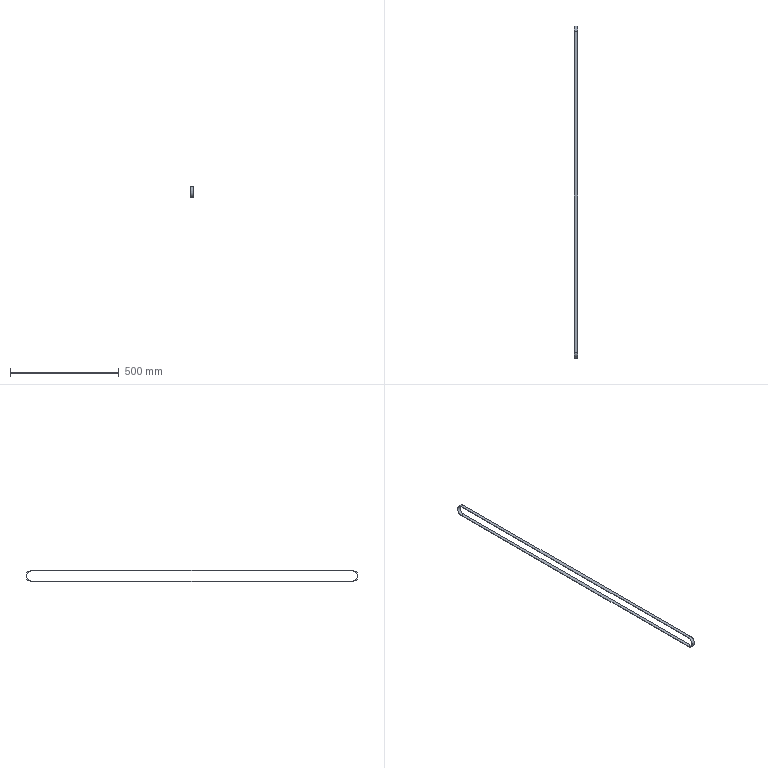Part | SolidWorks | features BaseBody 1 | 1 solid | 10 faces | box 15 x 1524 x 50.9 mm | volume 92989 mm3 | plane 6 | cylinder 4 | commonest cylinder face diameters 46.9 x2 50.9 x2
STEP:
#1=CARTESIAN_POINT('',(32.847,1932.,-322.55));
#2=VERTEX_POINT('',#1);
#3=CARTESIAN_POINT('',(32.847,459.,-322.55));
#4=VERTEX_POINT('',#3);
#5=CARTESIAN_POINT('',(32.847,1982.,-322.55));
#6=DIRECTION('',(0.,-1.,0.));
#7=VECTOR('',#6,1000.);
#8=LINE('',#5,#7);
#9=EDGE_CURVE('',#2,#4,#8,.T.);
#10=ORIENTED_EDGE('',*,*,#9,.F.);
#11=CARTESIAN_POINT('',(17.847,1932.,-322.55));
#12=VERTEX_POINT('',#11);
#13=CARTESIAN_POINT('',(32.847,1932.,-322.55));
#14=DIRECTION('',(1.,0.,0.));
#15=VECTOR('',#14,1000.);
#16=LINE('',#13,#15);
#17=EDGE_CURVE('',#12,#2,#16,.T.);
#18=ORIENTED_EDGE('',*,*,#17,.F.);
#19=CARTESIAN_POINT('',(17.847,459.,-322.55));
#20=VERTEX_POINT('',#19);
#21=CARTESIAN_POINT('',(17.847,1982.,-322.55));
#22=DIRECTION('',(0.,1.,0.));
#23=VECTOR('',#22,1000.);
#24=LINE('',#21,#23);
#25=EDGE_CURVE('',#20,#12,#24,.T.);
#26=ORIENTED_EDGE('',*,*,#25,.F.);
#27=CARTESIAN_POINT('',(32.847,459.,-322.55));
#28=DIRECTION('',(-1.,0.,0.));
#29=VECTOR('',#28,1000.);
#30=LINE('',#27,#29);
#31=EDGE_CURVE('',#4,#20,#30,.T.);
#32=ORIENTED_EDGE('',*,*,#31,.F.);
#33=EDGE_LOOP('',(#10,#18,#26,#32));
#34=FACE_OUTER_BOUND('',#33,.T.);
#35=CARTESIAN_POINT('',(32.847,1982.,-322.55));
#36=DIRECTION('',(0.,0.,-1.));
#37=DIRECTION('',(-1.,0.,0.));
#38=AXIS2_PLACEMENT_3D('',#35,#36,#37);
#39=PLANE('',#38);
#40=ADVANCED_FACE('',(#34),#39,.F.);
#41=ORIENTED_EDGE('',*,*,#31,.T.);
#42=CARTESIAN_POINT('',(17.847,459.,-373.45));
#43=VERTEX_POINT('',#42);
#44=CARTESIAN_POINT('',(17.847,459.,-348.));
#45=DIRECTION('',(1.,0.,0.));
#46=DIRECTION('',(0.,0.,1.));
#47=AXIS2_PLACEMENT_3D('',#44,#45,#46);
#48=CIRCLE('',#47,25.45);
#49=EDGE_CURVE('',#20,#43,#48,.T.);
#50=ORIENTED_EDGE('',*,*,#49,.T.);
#51=CARTESIAN_POINT('',(32.847,459.,-373.45));
#52=VERTEX_POINT('',#51);
#53=CARTESIAN_POINT('',(32.847,459.,-373.45));
#54=DIRECTION('',(1.,0.,0.));
#55=VECTOR('',#54,1000.);
#56=LINE('',#53,#55);
#57=EDGE_CURVE('',#43,#52,#56,.T.);
#58=ORIENTED_EDGE('',*,*,#57,.T.);
#59=CARTESIAN_POINT('',(32.847,459.,-348.));
#60=DIRECTION('',(-1.,0.,0.));
#61=DIRECTION('',(0.,0.,1.));
#62=AXIS2_PLACEMENT_3D('',#59,#60,#61);
#63=CIRCLE('',#62,25.45);
#64=EDGE_CURVE('',#52,#4,#63,.T.);
#65=ORIENTED_EDGE('',*,*,#64,.T.);
#66=EDGE_LOOP('',(#41,#50,#58,#65));
#67=FACE_OUTER_BOUND('',#66,.T.);
#68=CARTESIAN_POINT('',(32.847,459.,-348.));
#69=DIRECTION('',(-1.,0.,0.));
#70=DIRECTION('',(0.,0.,1.));
#71=AXIS2_PLACEMENT_3D('',#68,#69,#70);
#72=CYLINDRICAL_SURFACE('',#71,25.45);
#73=ADVANCED_FACE('',(#67),#72,.T.);
#74=CARTESIAN_POINT('',(32.847,459.,-371.45));
#75=VERTEX_POINT('',#74);
#76=CARTESIAN_POINT('',(32.847,1932.,-371.45));
#77=VERTEX_POINT('',#76);
#78=CARTESIAN_POINT('',(32.847,1982.,-371.45));
#79=DIRECTION('',(0.,1.,0.));
#80=VECTOR('',#79,1000.);
#81=LINE('',#78,#80);
#82=EDGE_CURVE('',#75,#77,#81,.T.);
#83=ORIENTED_EDGE('',*,*,#82,.F.);
#84=CARTESIAN_POINT('',(32.847,459.,-324.55));
#85=VERTEX_POINT('',#84);
#86=CARTESIAN_POINT('',(32.847,459.,-348.));
#87=DIRECTION('',(1.,0.,0.));
#88=DIRECTION('',(0.,0.,1.));
#89=AXIS2_PLACEMENT_3D('',#86,#87,#88);
#90=CIRCLE('',#89,23.45);
#91=EDGE_CURVE('',#85,#75,#90,.T.);
#92=ORIENTED_EDGE('',*,*,#91,.F.);
#93=CARTESIAN_POINT('',(32.847,1932.,-324.55));
#94=VERTEX_POINT('',#93);
#95=CARTESIAN_POINT('',(32.847,1982.,-324.55));
#96=DIRECTION('',(0.,-1.,0.));
#97=VECTOR('',#96,1000.);
#98=LINE('',#95,#97);
#99=EDGE_CURVE('',#94,#85,#98,.T.);
#100=ORIENTED_EDGE('',*,*,#99,.F.);
#101=CARTESIAN_POINT('',(32.847,1932.,-348.));
#102=DIRECTION('',(1.,0.,0.));
#103=DIRECTION('',(0.,0.,1.));
#104=AXIS2_PLACEMENT_3D('',#101,#102,#103);
#105=CIRCLE('',#104,23.45);
#106=EDGE_CURVE('',#77,#94,#105,.T.);
#107=ORIENTED_EDGE('',*,*,#106,.F.);
#108=EDGE_LOOP('',(#83,#92,#100,#107));
#109=FACE_BOUND('',#108,.T.);
#110=ORIENTED_EDGE('',*,*,#9,.T.);
#111=ORIENTED_EDGE('',*,*,#64,.F.);
#112=CARTESIAN_POINT('',(32.847,1932.,-373.45));
#113=VERTEX_POINT('',#112);
#114=CARTESIAN_POINT('',(32.847,1982.,-373.45));
#115=DIRECTION('',(0.,-1.,0.));
#116=VECTOR('',#115,1000.);
#117=LINE('',#114,#116);
#118=EDGE_CURVE('',#113,#52,#117,.T.);
#119=ORIENTED_EDGE('',*,*,#118,.F.);
#120=CARTESIAN_POINT('',(32.847,1932.,-348.));
#121=DIRECTION('',(-1.,0.,0.));
#122=DIRECTION('',(0.,0.,1.));
#123=AXIS2_PLACEMENT_3D('',#120,#121,#122);
#124=CIRCLE('',#123,25.45);
#125=EDGE_CURVE('',#2,#113,#124,.T.);
#126=ORIENTED_EDGE('',*,*,#125,.F.);
#127=EDGE_LOOP('',(#110,#111,#119,#126));
#128=FACE_OUTER_BOUND('',#127,.T.);
#129=CARTESIAN_POINT('',(32.847,1982.,-348.));
#130=DIRECTION('',(-1.,0.,0.));
#131=DIRECTION('',(0.,0.,1.));
#132=AXIS2_PLACEMENT_3D('',#129,#130,#131);
#133=PLANE('',#132);
#134=ADVANCED_FACE('',(#109,#128),#133,.F.);
#135=CARTESIAN_POINT('',(17.847,1932.,-373.45));
#136=VERTEX_POINT('',#135);
#137=CARTESIAN_POINT('',(32.847,1932.,-373.45));
#138=DIRECTION('',(-1.,0.,0.));
#139=VECTOR('',#138,1000.);
#140=LINE('',#137,#139);
#141=EDGE_CURVE('',#113,#136,#140,.T.);
#142=ORIENTED_EDGE('',*,*,#141,.T.);
#143=CARTESIAN_POINT('',(17.847,1932.,-348.));
#144=DIRECTION('',(1.,0.,0.));
#145=DIRECTION('',(0.,0.,1.));
#146=AXIS2_PLACEMENT_3D('',#143,#144,#145);
#147=CIRCLE('',#146,25.45);
#148=EDGE_CURVE('',#136,#12,#147,.T.);
#149=ORIENTED_EDGE('',*,*,#148,.T.);
#150=ORIENTED_EDGE('',*,*,#17,.T.);
#151=ORIENTED_EDGE('',*,*,#125,.T.);
#152=EDGE_LOOP('',(#142,#149,#150,#151));
#153=FACE_OUTER_BOUND('',#152,.T.);
#154=CARTESIAN_POINT('',(32.847,1932.,-348.));
#155=DIRECTION('',(-1.,0.,0.));
#156=DIRECTION('',(0.,0.,1.));
#157=AXIS2_PLACEMENT_3D('',#154,#155,#156);
#158=CYLINDRICAL_SURFACE('',#157,25.45);
#159=ADVANCED_FACE('',(#153),#158,.T.);
#160=CARTESIAN_POINT('',(17.847,459.,-324.55));
#161=VERTEX_POINT('',#160);
#162=CARTESIAN_POINT('',(17.847,459.,-371.45));
#163=VERTEX_POINT('',#162);
#164=CARTESIAN_POINT('',(17.847,459.,-348.));
#165=DIRECTION('',(1.,0.,0.));
#166=DIRECTION('',(0.,0.,1.));
#167=AXIS2_PLACEMENT_3D('',#164,#165,#166);
#168=CIRCLE('',#167,23.45);
#169=EDGE_CURVE('',#161,#163,#168,.T.);
#170=ORIENTED_EDGE('',*,*,#169,.T.);
#171=CARTESIAN_POINT('',(17.847,1932.,-371.45));
#172=VERTEX_POINT('',#171);
#173=CARTESIAN_POINT('',(17.847,1982.,-371.45));
#174=DIRECTION('',(0.,1.,0.));
#175=VECTOR('',#174,1000.);
#176=LINE('',#173,#175);
#177=EDGE_CURVE('',#163,#172,#176,.T.);
#178=ORIENTED_EDGE('',*,*,#177,.T.);
#179=CARTESIAN_POINT('',(17.847,1932.,-324.55));
#180=VERTEX_POINT('',#179);
#181=CARTESIAN_POINT('',(17.847,1932.,-348.));
#182=DIRECTION('',(1.,0.,0.));
#183=DIRECTION('',(0.,0.,1.));
#184=AXIS2_PLACEMENT_3D('',#181,#182,#183);
#185=CIRCLE('',#184,23.45);
#186=EDGE_CURVE('',#172,#180,#185,.T.);
#187=ORIENTED_EDGE('',*,*,#186,.T.);
#188=CARTESIAN_POINT('',(17.847,1982.,-324.55));
#189=DIRECTION('',(0.,-1.,0.));
#190=VECTOR('',#189,1000.);
#191=LINE('',#188,#190);
#192=EDGE_CURVE('',#180,#161,#191,.T.);
#193=ORIENTED_EDGE('',*,*,#192,.T.);
#194=EDGE_LOOP('',(#170,#178,#187,#193));
#195=FACE_BOUND('',#194,.T.);
#196=ORIENTED_EDGE('',*,*,#25,.T.);
#197=ORIENTED_EDGE('',*,*,#148,.F.);
#198=CARTESIAN_POINT('',(17.847,1982.,-373.45));
#199=DIRECTION('',(0.,-1.,0.));
#200=VECTOR('',#199,1000.);
#201=LINE('',#198,#200);
#202=EDGE_CURVE('',#136,#43,#201,.T.);
#203=ORIENTED_EDGE('',*,*,#202,.T.);
#204=ORIENTED_EDGE('',*,*,#49,.F.);
#205=EDGE_LOOP('',(#196,#197,#203,#204));
#206=FACE_OUTER_BOUND('',#205,.T.);
#207=CARTESIAN_POINT('',(17.847,1982.,-348.));
#208=DIRECTION('',(-1.,0.,0.));
#209=DIRECTION('',(0.,0.,1.));
#210=AXIS2_PLACEMENT_3D('',#207,#208,#209);
#211=PLANE('',#210);
#212=ADVANCED_FACE('',(#195,#206),#211,.T.);
#213=ORIENTED_EDGE('',*,*,#118,.T.);
#214=ORIENTED_EDGE('',*,*,#57,.F.);
#215=ORIENTED_EDGE('',*,*,#202,.F.);
#216=ORIENTED_EDGE('',*,*,#141,.F.);
#217=EDGE_LOOP('',(#213,#214,#215,#216));
#218=FACE_OUTER_BOUND('',#217,.T.);
#219=CARTESIAN_POINT('',(32.847,1982.,-373.45));
#220=DIRECTION('',(0.,0.,1.));
#221=DIRECTION('',(1.,0.,0.));
#222=AXIS2_PLACEMENT_3D('',#219,#220,#221);
#223=PLANE('',#222);
#224=ADVANCED_FACE('',(#218),#223,.F.);
#225=CARTESIAN_POINT('',(32.847,1932.,-371.45));
#226=DIRECTION('',(-1.,0.,0.));
#227=VECTOR('',#226,1000.);
#228=LINE('',#225,#227);
#229=EDGE_CURVE('',#77,#172,#228,.T.);
#230=ORIENTED_EDGE('',*,*,#229,.F.);
#231=ORIENTED_EDGE('',*,*,#106,.T.);
#232=CARTESIAN_POINT('',(32.847,1932.,-324.55));
#233=DIRECTION('',(1.,0.,0.));
#234=VECTOR('',#233,1000.);
#235=LINE('',#232,#234);
#236=EDGE_CURVE('',#180,#94,#235,.T.);
#237=ORIENTED_EDGE('',*,*,#236,.F.);
#238=ORIENTED_EDGE('',*,*,#186,.F.);
#239=EDGE_LOOP('',(#230,#231,#237,#238));
#240=FACE_OUTER_BOUND('',#239,.T.);
#241=CARTESIAN_POINT('',(32.847,1932.,-348.));
#242=DIRECTION('',(-1.,0.,0.));
#243=DIRECTION('',(0.,0.,1.));
#244=AXIS2_PLACEMENT_3D('',#241,#242,#243);
#245=CYLINDRICAL_SURFACE('',#244,23.45);
#246=ADVANCED_FACE('',(#240),#245,.F.);
#247=ORIENTED_EDGE('',*,*,#229,.T.);
#248=ORIENTED_EDGE('',*,*,#177,.F.);
#249=CARTESIAN_POINT('',(32.847,459.,-371.45));
#250=DIRECTION('',(1.,0.,0.));
#251=VECTOR('',#250,1000.);
#252=LINE('',#249,#251);
#253=EDGE_CURVE('',#163,#75,#252,.T.);
#254=ORIENTED_EDGE('',*,*,#253,.T.);
#255=ORIENTED_EDGE('',*,*,#82,.T.);
#256=EDGE_LOOP('',(#247,#248,#254,#255));
#257=FACE_OUTER_BOUND('',#256,.T.);
#258=CARTESIAN_POINT('',(32.847,1982.,-371.45));
#259=DIRECTION('',(0.,0.,1.));
#260=DIRECTION('',(1.,0.,0.));
#261=AXIS2_PLACEMENT_3D('',#258,#259,#260);
#262=PLANE('',#261);
#263=ADVANCED_FACE('',(#257),#262,.T.);
#264=ORIENTED_EDGE('',*,*,#91,.T.);
#265=ORIENTED_EDGE('',*,*,#253,.F.);
#266=ORIENTED_EDGE('',*,*,#169,.F.);
#267=CARTESIAN_POINT('',(32.847,459.,-324.55));
#268=DIRECTION('',(-1.,0.,0.));
#269=VECTOR('',#268,1000.);
#270=LINE('',#267,#269);
#271=EDGE_CURVE('',#85,#161,#270,.T.);
#272=ORIENTED_EDGE('',*,*,#271,.F.);
#273=EDGE_LOOP('',(#264,#265,#266,#272));
#274=FACE_OUTER_BOUND('',#273,.T.);
#275=CARTESIAN_POINT('',(32.847,459.,-348.));
#276=DIRECTION('',(-1.,0.,0.));
#277=DIRECTION('',(0.,0.,1.));
#278=AXIS2_PLACEMENT_3D('',#275,#276,#277);
#279=CYLINDRICAL_SURFACE('',#278,23.45);
#280=ADVANCED_FACE('',(#274),#279,.F.);
#281=ORIENTED_EDGE('',*,*,#271,.T.);
#282=ORIENTED_EDGE('',*,*,#192,.F.);
#283=ORIENTED_EDGE('',*,*,#236,.T.);
#284=ORIENTED_EDGE('',*,*,#99,.T.);
#285=EDGE_LOOP('',(#281,#282,#283,#284));
#286=FACE_OUTER_BOUND('',#285,.T.);
#287=CARTESIAN_POINT('',(32.847,797.,-324.55));
#288=DIRECTION('',(0.,0.,-1.));
#289=DIRECTION('',(-1.,0.,0.));
#290=AXIS2_PLACEMENT_3D('',#287,#288,#289);
#291=PLANE('',#290);
#292=ADVANCED_FACE('',(#286),#291,.T.);
#293=CLOSED_SHELL('',(#40,#73,#134,#159,#212,#224,#246,#263,#280,#292));
#294=MANIFOLD_SOLID_BREP('',#293);
#295=CARTESIAN_POINT('',(0.,0.,0.));
#296=DIRECTION('',(0.,0.,1.));
#297=DIRECTION('',(1.,0.,0.));
#298=AXIS2_PLACEMENT_3D('',#295,#296,#297);
#299=(LENGTH_UNIT()NAMED_UNIT(*)SI_UNIT(.MILLI.,.METRE.));
#300=UNCERTAINTY_MEASURE_WITH_UNIT(LENGTH_MEASURE(0.00001),#299,'','');
#301=(NAMED_UNIT(*)PLANE_ANGLE_UNIT()SI_UNIT($,.RADIAN.));
#302=(NAMED_UNIT(*)SI_UNIT($,.STERADIAN.)SOLID_ANGLE_UNIT());
#303=(GEOMETRIC_REPRESENTATION_CONTEXT(3)GLOBAL_UNCERTAINTY_ASSIGNED_CONTEXT((#300))GLOBAL_UNIT_ASSIGNED_CONTEXT((#299,#301,#302))REPRESENTATION_CONTEXT('',''));
#304=ADVANCED_BREP_SHAPE_REPRESENTATION('',(#294,#298),#303);